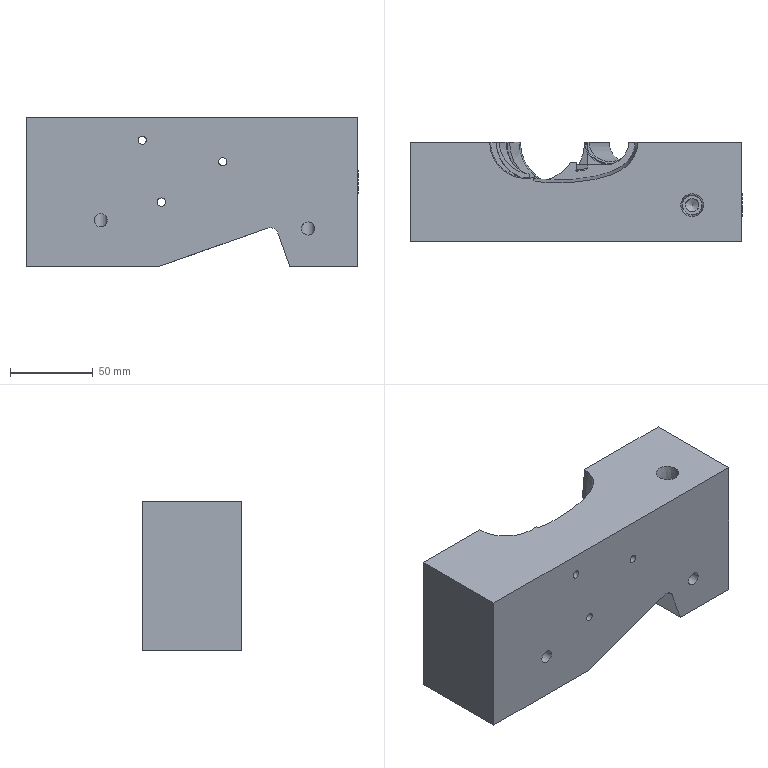Part | STEP file | COR_id646_x_t | 1 solid | 115 faces | box 200 x 60 x 90 mm | volume 873749 mm3 | plane 39 | cylinder 37 | other 21 | cone 10 | spline 8 | commonest cylinder face diameters 8 x7 1.934 x5 2.036 x4 1.018 x3 5 x3 59.553 x2